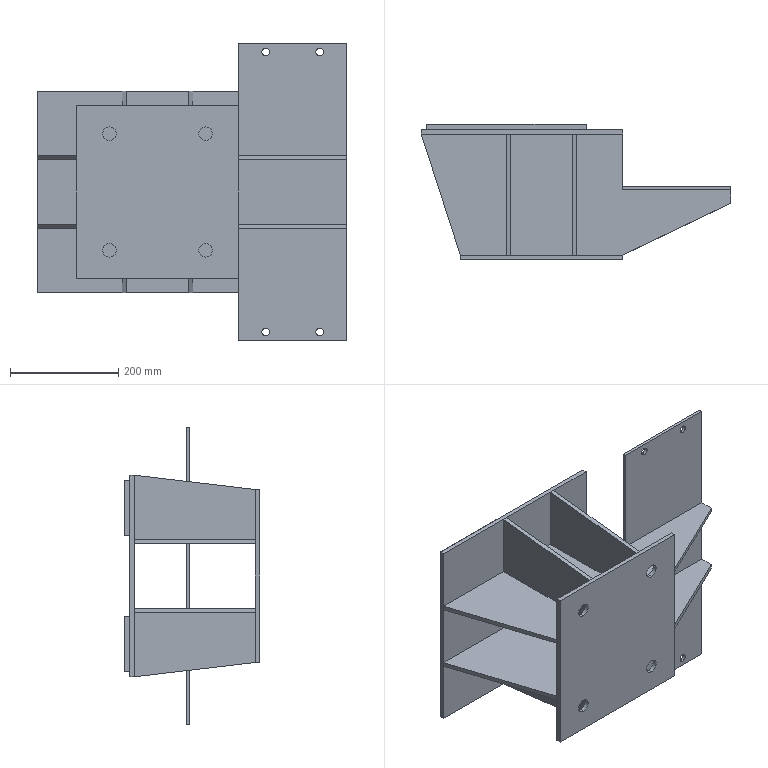Part | STEP file | Motor base_Default<As machined> | 11 solids | 88 faces | box 572.5 x 250 x 550 mm | volume 5315088 mm3 | plane 72 | cylinder 16 | commonest cylinder face diameters 14 x8 25 x8